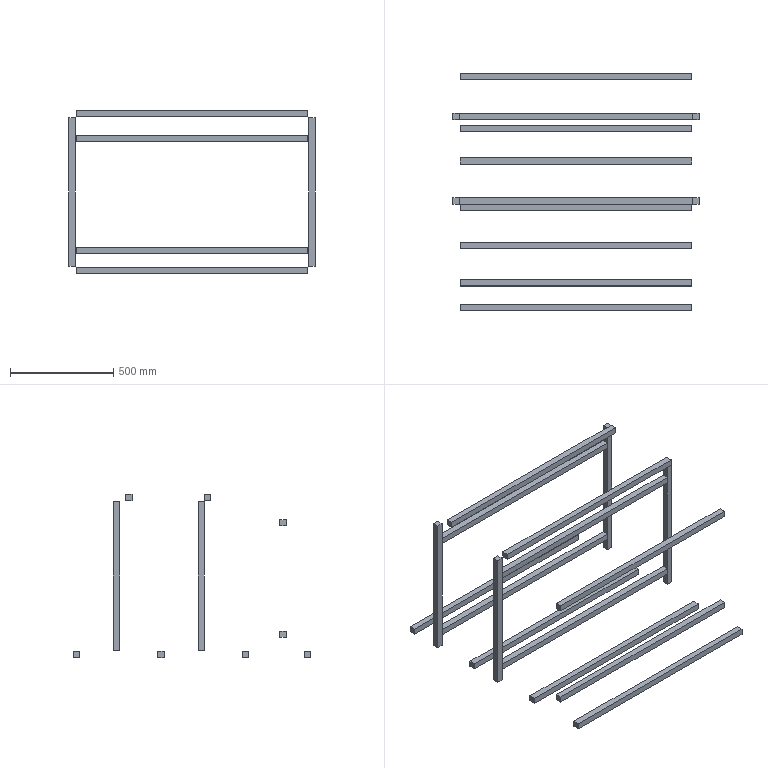Part | SolidWorks | features BaseBody 16 | 16 solids | 96 faces | box 1190 x 1150 x 790 mm | volume 14724000 mm3 | plane 96